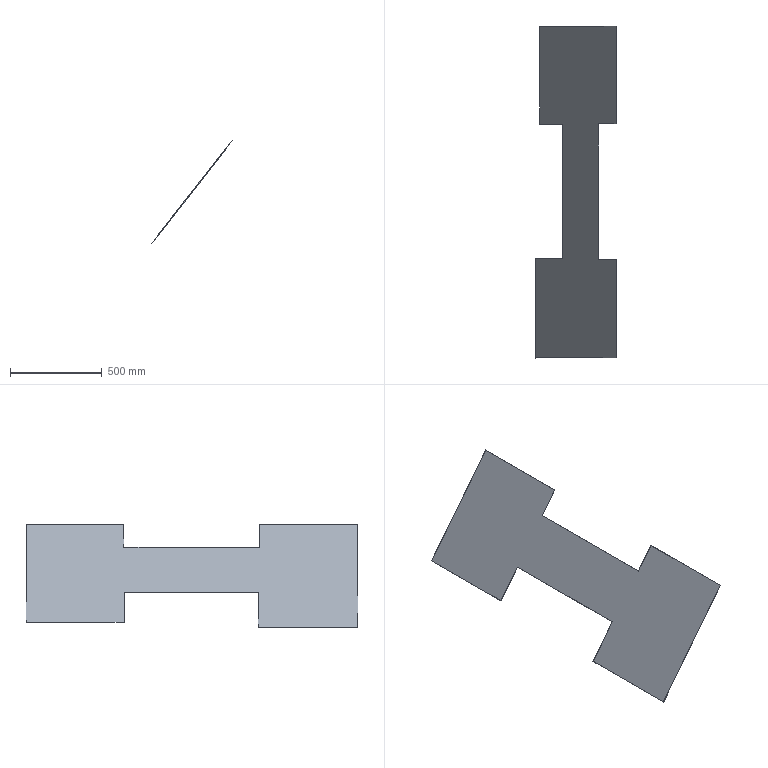Part | STEP file | fixed baffle panel | 1 solid | 14 faces | box 439.017 x 1805 x 559.044 mm | volume 1940108 mm3 | plane 14
STEP:
#1=CARTESIAN_POINT('',(0.,0.,0.));
#2=DIRECTION('',(0.,0.,1.));
#3=DIRECTION('',(1.,0.,0.));
#4=AXIS2_PLACEMENT_3D('',#1,#2,#3);
#5=CARTESIAN_POINT('',(962.42,-360.483,12.039));
#6=VERTEX_POINT('',#5);
#7=CARTESIAN_POINT('',(962.42,-902.,12.039));
#8=VERTEX_POINT('',#7);
#9=CARTESIAN_POINT('',(962.42,-360.483,12.039));
#10=DIRECTION('',(0.,-1.,0.));
#11=VECTOR('',#10,1.);
#12=LINE('',#9,#11);
#13=CARTESIAN_POINT('',(963.994,-360.483,10.805));
#14=DIRECTION('',(-0.6171,0.,-0.7869));
#15=DIRECTION('',(0.7869,0.,-0.6171));
#16=AXIS2_PLACEMENT_3D('',#13,#14,#15);
#17=PLANE('',#16);
#18=CARTESIAN_POINT('',(-2.,0.));
#19=DIRECTION('',(0.,1.));
#20=VECTOR('',#19,1.);
#21=LINE('',#18,#20);
#22=(GEOMETRIC_REPRESENTATION_CONTEXT(2)PARAMETRIC_REPRESENTATION_CONTEXT()REPRESENTATION_CONTEXT('',''));
#23=DEFINITIONAL_REPRESENTATION('',(#21),#22);
#24=PCURVE('',#17,#23);
#25=CARTESIAN_POINT('',(590.082,0.,-462.752));
#26=DIRECTION('',(-0.7869,0.,0.6171));
#27=DIRECTION('',(-0.6171,0.,-0.7869));
#28=AXIS2_PLACEMENT_3D('',#25,#26,#27);
#29=PLANE('',#28);
#30=CARTESIAN_POINT('',(-603.376,360.483));
#31=DIRECTION('',(0.,1.));
#32=VECTOR('',#31,1.);
#33=LINE('',#30,#32);
#34=(GEOMETRIC_REPRESENTATION_CONTEXT(2)PARAMETRIC_REPRESENTATION_CONTEXT()REPRESENTATION_CONTEXT('',''));
#35=DEFINITIONAL_REPRESENTATION('',(#33),#34);
#36=PCURVE('',#29,#35);
#37=SURFACE_CURVE('',#12,(#24,#36),.PCURVE_S1.);
#38=EDGE_CURVE('',#6,#8,#37,.T.);
#39=ORIENTED_EDGE('',*,*,#38,.F.);
#40=CARTESIAN_POINT('',(963.994,-360.483,10.805));
#41=VERTEX_POINT('',#40);
#42=CARTESIAN_POINT('',(963.994,-360.483,10.805));
#43=DIRECTION('',(-0.7869,0.,0.6171));
#44=VECTOR('',#43,1.);
#45=LINE('',#42,#44);
#46=CARTESIAN_POINT('',(0.,0.));
#47=DIRECTION('',(-1.,0.));
#48=VECTOR('',#47,1.);
#49=LINE('',#46,#48);
#50=(GEOMETRIC_REPRESENTATION_CONTEXT(2)PARAMETRIC_REPRESENTATION_CONTEXT()REPRESENTATION_CONTEXT('',''));
#51=DEFINITIONAL_REPRESENTATION('',(#49),#50);
#52=PCURVE('',#17,#51);
#53=CARTESIAN_POINT('',(1112.096,-360.483,199.658));
#54=DIRECTION('',(0.,1.,0.));
#55=DIRECTION('',(0.,0.,-1.));
#56=AXIS2_PLACEMENT_3D('',#53,#54,#55);
#57=PLANE('',#56);
#58=CARTESIAN_POINT('',(188.854,148.102));
#59=DIRECTION('',(-0.6171,0.7869));
#60=VECTOR('',#59,1.);
#61=LINE('',#58,#60);
#62=(GEOMETRIC_REPRESENTATION_CONTEXT(2)PARAMETRIC_REPRESENTATION_CONTEXT()REPRESENTATION_CONTEXT('',''));
#63=DEFINITIONAL_REPRESENTATION('',(#61),#62);
#64=PCURVE('',#57,#63);
#65=SURFACE_CURVE('',#45,(#52,#64),.PCURVE_S1.);
#66=EDGE_CURVE('',#41,#6,#65,.T.);
#67=ORIENTED_EDGE('',*,*,#66,.F.);
#68=CARTESIAN_POINT('',(963.994,-902.,10.805));
#69=VERTEX_POINT('',#68);
#70=CARTESIAN_POINT('',(963.994,-360.483,10.805));
#71=DIRECTION('',(0.,-1.,0.));
#72=VECTOR('',#71,1.);
#73=LINE('',#70,#72);
#74=CARTESIAN_POINT('',(0.,0.));
#75=DIRECTION('',(0.,1.));
#76=VECTOR('',#75,1.);
#77=LINE('',#74,#76);
#78=(GEOMETRIC_REPRESENTATION_CONTEXT(2)PARAMETRIC_REPRESENTATION_CONTEXT()REPRESENTATION_CONTEXT('',''));
#79=DEFINITIONAL_REPRESENTATION('',(#77),#78);
#80=PCURVE('',#17,#79);
#81=CARTESIAN_POINT('',(591.655,0.,-463.986));
#82=DIRECTION('',(-0.7869,0.,0.6171));
#83=DIRECTION('',(-0.6171,0.,-0.7869));
#84=AXIS2_PLACEMENT_3D('',#81,#82,#83);
#85=PLANE('',#84);
#86=CARTESIAN_POINT('',(-603.376,360.483));
#87=DIRECTION('',(0.,1.));
#88=VECTOR('',#87,1.);
#89=LINE('',#86,#88);
#90=(GEOMETRIC_REPRESENTATION_CONTEXT(2)PARAMETRIC_REPRESENTATION_CONTEXT()REPRESENTATION_CONTEXT('',''));
#91=DEFINITIONAL_REPRESENTATION('',(#89),#90);
#92=PCURVE('',#85,#91);
#93=SURFACE_CURVE('',#73,(#80,#92),.PCURVE_S1.);
#94=EDGE_CURVE('',#41,#69,#93,.T.);
#95=ORIENTED_EDGE('',*,*,#94,.T.);
#96=CARTESIAN_POINT('',(963.994,-902.,10.805));
#97=DIRECTION('',(-0.7869,0.,0.6171));
#98=VECTOR('',#97,1.);
#99=LINE('',#96,#98);
#100=CARTESIAN_POINT('',(0.,541.517));
#101=DIRECTION('',(-1.,0.));
#102=VECTOR('',#101,1.);
#103=LINE('',#100,#102);
#104=(GEOMETRIC_REPRESENTATION_CONTEXT(2)PARAMETRIC_REPRESENTATION_CONTEXT()REPRESENTATION_CONTEXT('',''));
#105=DEFINITIONAL_REPRESENTATION('',(#103),#104);
#106=PCURVE('',#17,#105);
#107=CARTESIAN_POINT('',(963.994,-902.,10.805));
#108=DIRECTION('',(0.,-1.,0.));
#109=DIRECTION('',(0.,0.,1.));
#110=AXIS2_PLACEMENT_3D('',#107,#108,#109);
#111=PLANE('',#110);
#112=CARTESIAN_POINT('',(0.,0.));
#113=DIRECTION('',(0.6171,0.7869));
#114=VECTOR('',#113,1.);
#115=LINE('',#112,#114);
#116=(GEOMETRIC_REPRESENTATION_CONTEXT(2)PARAMETRIC_REPRESENTATION_CONTEXT()REPRESENTATION_CONTEXT('',''));
#117=DEFINITIONAL_REPRESENTATION('',(#115),#116);
#118=PCURVE('',#111,#117);
#119=SURFACE_CURVE('',#99,(#106,#118),.PCURVE_S1.);
#120=EDGE_CURVE('',#69,#8,#119,.T.);
#121=ORIENTED_EDGE('',*,*,#120,.T.);
#122=EDGE_LOOP('',(#39,#67,#95,#121));
#123=FACE_BOUND('',#122,.T.);
#124=ADVANCED_FACE('',(#123),#17,.T.);
#125=CARTESIAN_POINT('',(1399.864,-902.,569.848));
#126=VERTEX_POINT('',#125);
#127=CARTESIAN_POINT('',(962.42,-902.,12.039));
#128=DIRECTION('',(0.6171,0.,0.7869));
#129=VECTOR('',#128,1.);
#130=LINE('',#127,#129);
#131=CARTESIAN_POINT('',(1.234,1.574));
#132=DIRECTION('',(0.7869,-0.6171));
#133=VECTOR('',#132,1.);
#134=LINE('',#131,#133);
#135=(GEOMETRIC_REPRESENTATION_CONTEXT(2)PARAMETRIC_REPRESENTATION_CONTEXT()REPRESENTATION_CONTEXT('',''));
#136=DEFINITIONAL_REPRESENTATION('',(#134),#135);
#137=PCURVE('',#111,#136);
#138=CARTESIAN_POINT('',(-603.376,902.));
#139=DIRECTION('',(-1.,0.));
#140=VECTOR('',#139,1.);
#141=LINE('',#138,#140);
#142=(GEOMETRIC_REPRESENTATION_CONTEXT(2)PARAMETRIC_REPRESENTATION_CONTEXT()REPRESENTATION_CONTEXT('',''));
#143=DEFINITIONAL_REPRESENTATION('',(#141),#142);
#144=PCURVE('',#29,#143);
#145=SURFACE_CURVE('',#130,(#137,#144),.PCURVE_S1.);
#146=EDGE_CURVE('',#8,#126,#145,.T.);
#147=ORIENTED_EDGE('',*,*,#146,.F.);
#148=ORIENTED_EDGE('',*,*,#120,.F.);
#149=CARTESIAN_POINT('',(1401.438,-902.,568.614));
#150=VERTEX_POINT('',#149);
#151=CARTESIAN_POINT('',(963.994,-902.,10.805));
#152=DIRECTION('',(0.6171,0.,0.7869));
#153=VECTOR('',#152,1.);
#154=LINE('',#151,#153);
#155=CARTESIAN_POINT('',(0.,0.));
#156=DIRECTION('',(0.7869,-0.6171));
#157=VECTOR('',#156,1.);
#158=LINE('',#155,#157);
#159=(GEOMETRIC_REPRESENTATION_CONTEXT(2)PARAMETRIC_REPRESENTATION_CONTEXT()REPRESENTATION_CONTEXT('',''));
#160=DEFINITIONAL_REPRESENTATION('',(#158),#159);
#161=PCURVE('',#111,#160);
#162=CARTESIAN_POINT('',(-603.376,902.));
#163=DIRECTION('',(-1.,0.));
#164=VECTOR('',#163,1.);
#165=LINE('',#162,#164);
#166=(GEOMETRIC_REPRESENTATION_CONTEXT(2)PARAMETRIC_REPRESENTATION_CONTEXT()REPRESENTATION_CONTEXT('',''));
#167=DEFINITIONAL_REPRESENTATION('',(#165),#166);
#168=PCURVE('',#85,#167);
#169=SURFACE_CURVE('',#154,(#161,#168),.PCURVE_S1.);
#170=EDGE_CURVE('',#69,#150,#169,.T.);
#171=ORIENTED_EDGE('',*,*,#170,.T.);
#172=CARTESIAN_POINT('',(1401.438,-902.,568.614));
#173=DIRECTION('',(-0.7869,0.,0.6171));
#174=VECTOR('',#173,1.);
#175=LINE('',#172,#174);
#176=CARTESIAN_POINT('',(557.809,-437.443));
#177=DIRECTION('',(0.6171,0.7869));
#178=VECTOR('',#177,1.);
#179=LINE('',#176,#178);
#180=(GEOMETRIC_REPRESENTATION_CONTEXT(2)PARAMETRIC_REPRESENTATION_CONTEXT()REPRESENTATION_CONTEXT('',''));
#181=DEFINITIONAL_REPRESENTATION('',(#179),#180);
#182=PCURVE('',#111,#181);
#183=CARTESIAN_POINT('',(1401.438,-902.,568.614));
#184=DIRECTION('',(0.6171,0.,0.7869));
#185=DIRECTION('',(-0.7869,0.,0.6171));
#186=AXIS2_PLACEMENT_3D('',#183,#184,#185);
#187=PLANE('',#186);
#188=CARTESIAN_POINT('',(0.,0.));
#189=DIRECTION('',(1.,0.));
#190=VECTOR('',#189,1.);
#191=LINE('',#188,#190);
#192=(GEOMETRIC_REPRESENTATION_CONTEXT(2)PARAMETRIC_REPRESENTATION_CONTEXT()REPRESENTATION_CONTEXT('',''));
#193=DEFINITIONAL_REPRESENTATION('',(#191),#192);
#194=PCURVE('',#187,#193);
#195=SURFACE_CURVE('',#175,(#182,#194),.PCURVE_S1.);
#196=EDGE_CURVE('',#150,#126,#195,.T.);
#197=ORIENTED_EDGE('',*,*,#196,.T.);
#198=EDGE_LOOP('',(#147,#148,#171,#197));
#199=FACE_BOUND('',#198,.T.);
#200=ADVANCED_FACE('',(#199),#111,.T.);
#201=CARTESIAN_POINT('',(1399.864,-368.483,569.848));
#202=VERTEX_POINT('',#201);
#203=CARTESIAN_POINT('',(1399.864,-902.,569.848));
#204=DIRECTION('',(0.,1.,0.));
#205=VECTOR('',#204,1.);
#206=LINE('',#203,#205);
#207=CARTESIAN_POINT('',(2.,0.));
#208=DIRECTION('',(0.,-1.));
#209=VECTOR('',#208,1.);
#210=LINE('',#207,#209);
#211=(GEOMETRIC_REPRESENTATION_CONTEXT(2)PARAMETRIC_REPRESENTATION_CONTEXT()REPRESENTATION_CONTEXT('',''));
#212=DEFINITIONAL_REPRESENTATION('',(#210),#211);
#213=PCURVE('',#187,#212);
#214=CARTESIAN_POINT('',(-1312.254,902.));
#215=DIRECTION('',(0.,-1.));
#216=VECTOR('',#215,1.);
#217=LINE('',#214,#216);
#218=(GEOMETRIC_REPRESENTATION_CONTEXT(2)PARAMETRIC_REPRESENTATION_CONTEXT()REPRESENTATION_CONTEXT('',''));
#219=DEFINITIONAL_REPRESENTATION('',(#217),#218);
#220=PCURVE('',#29,#219);
#221=SURFACE_CURVE('',#206,(#213,#220),.PCURVE_S1.);
#222=EDGE_CURVE('',#126,#202,#221,.T.);
#223=ORIENTED_EDGE('',*,*,#222,.F.);
#224=ORIENTED_EDGE('',*,*,#196,.F.);
#225=CARTESIAN_POINT('',(1401.438,-368.483,568.614));
#226=VERTEX_POINT('',#225);
#227=CARTESIAN_POINT('',(1401.438,-902.,568.614));
#228=DIRECTION('',(0.,1.,0.));
#229=VECTOR('',#228,1.);
#230=LINE('',#227,#229);
#231=CARTESIAN_POINT('',(0.,0.));
#232=DIRECTION('',(0.,-1.));
#233=VECTOR('',#232,1.);
#234=LINE('',#231,#233);
#235=(GEOMETRIC_REPRESENTATION_CONTEXT(2)PARAMETRIC_REPRESENTATION_CONTEXT()REPRESENTATION_CONTEXT('',''));
#236=DEFINITIONAL_REPRESENTATION('',(#234),#235);
#237=PCURVE('',#187,#236);
#238=CARTESIAN_POINT('',(-1312.254,902.));
#239=DIRECTION('',(0.,-1.));
#240=VECTOR('',#239,1.);
#241=LINE('',#238,#240);
#242=(GEOMETRIC_REPRESENTATION_CONTEXT(2)PARAMETRIC_REPRESENTATION_CONTEXT()REPRESENTATION_CONTEXT('',''));
#243=DEFINITIONAL_REPRESENTATION('',(#241),#242);
#244=PCURVE('',#85,#243);
#245=SURFACE_CURVE('',#230,(#237,#244),.PCURVE_S1.);
#246=EDGE_CURVE('',#150,#226,#245,.T.);
#247=ORIENTED_EDGE('',*,*,#246,.T.);
#248=CARTESIAN_POINT('',(1401.438,-368.483,568.614));
#249=DIRECTION('',(-0.7869,0.,0.6171));
#250=VECTOR('',#249,1.);
#251=LINE('',#248,#250);
#252=CARTESIAN_POINT('',(0.,-533.517));
#253=DIRECTION('',(1.,0.));
#254=VECTOR('',#253,1.);
#255=LINE('',#252,#254);
#256=(GEOMETRIC_REPRESENTATION_CONTEXT(2)PARAMETRIC_REPRESENTATION_CONTEXT()REPRESENTATION_CONTEXT('',''));
#257=DEFINITIONAL_REPRESENTATION('',(#255),#256);
#258=PCURVE('',#187,#257);
#259=CARTESIAN_POINT('',(1401.438,-368.483,568.614));
#260=DIRECTION('',(0.,1.,0.));
#261=DIRECTION('',(0.,0.,-1.));
#262=AXIS2_PLACEMENT_3D('',#259,#260,#261);
#263=PLANE('',#262);
#264=CARTESIAN_POINT('',(0.,0.));
#265=DIRECTION('',(-0.6171,0.7869));
#266=VECTOR('',#265,1.);
#267=LINE('',#264,#266);
#268=(GEOMETRIC_REPRESENTATION_CONTEXT(2)PARAMETRIC_REPRESENTATION_CONTEXT()REPRESENTATION_CONTEXT('',''));
#269=DEFINITIONAL_REPRESENTATION('',(#267),#268);
#270=PCURVE('',#263,#269);
#271=SURFACE_CURVE('',#251,(#258,#270),.PCURVE_S1.);
#272=EDGE_CURVE('',#226,#202,#271,.T.);
#273=ORIENTED_EDGE('',*,*,#272,.T.);
#274=EDGE_LOOP('',(#223,#224,#247,#273));
#275=FACE_BOUND('',#274,.T.);
#276=ADVANCED_FACE('',(#275),#187,.T.);
#277=CARTESIAN_POINT('',(1303.535,-368.483,447.013));
#278=VERTEX_POINT('',#277);
#279=CARTESIAN_POINT('',(1399.864,-368.483,569.848));
#280=DIRECTION('',(-0.6171,0.,-0.7869));
#281=VECTOR('',#280,1.);
#282=LINE('',#279,#281);
#283=CARTESIAN_POINT('',(-1.234,1.574));
#284=DIRECTION('',(0.7869,0.6171));
#285=VECTOR('',#284,1.);
#286=LINE('',#283,#285);
#287=(GEOMETRIC_REPRESENTATION_CONTEXT(2)PARAMETRIC_REPRESENTATION_CONTEXT()REPRESENTATION_CONTEXT('',''));
#288=DEFINITIONAL_REPRESENTATION('',(#286),#287);
#289=PCURVE('',#263,#288);
#290=CARTESIAN_POINT('',(-1312.254,368.483));
#291=DIRECTION('',(1.,0.));
#292=VECTOR('',#291,1.);
#293=LINE('',#290,#292);
#294=(GEOMETRIC_REPRESENTATION_CONTEXT(2)PARAMETRIC_REPRESENTATION_CONTEXT()REPRESENTATION_CONTEXT('',''));
#295=DEFINITIONAL_REPRESENTATION('',(#293),#294);
#296=PCURVE('',#29,#295);
#297=SURFACE_CURVE('',#282,(#289,#296),.PCURVE_S1.);
#298=EDGE_CURVE('',#202,#278,#297,.T.);
#299=ORIENTED_EDGE('',*,*,#298,.F.);
#300=ORIENTED_EDGE('',*,*,#272,.F.);
#301=CARTESIAN_POINT('',(1305.108,-368.483,445.779));
#302=VERTEX_POINT('',#301);
#303=CARTESIAN_POINT('',(1401.438,-368.483,568.614));
#304=DIRECTION('',(-0.6171,0.,-0.7869));
#305=VECTOR('',#304,1.);
#306=LINE('',#303,#305);
#307=CARTESIAN_POINT('',(0.,0.));
#308=DIRECTION('',(0.7869,0.6171));
#309=VECTOR('',#308,1.);
#310=LINE('',#307,#309);
#311=(GEOMETRIC_REPRESENTATION_CONTEXT(2)PARAMETRIC_REPRESENTATION_CONTEXT()REPRESENTATION_CONTEXT('',''));
#312=DEFINITIONAL_REPRESENTATION('',(#310),#311);
#313=PCURVE('',#263,#312);
#314=CARTESIAN_POINT('',(-1312.254,368.483));
#315=DIRECTION('',(1.,0.));
#316=VECTOR('',#315,1.);
#317=LINE('',#314,#316);
#318=(GEOMETRIC_REPRESENTATION_CONTEXT(2)PARAMETRIC_REPRESENTATION_CONTEXT()REPRESENTATION_CONTEXT('',''));
#319=DEFINITIONAL_REPRESENTATION('',(#317),#318);
#320=PCURVE('',#85,#319);
#321=SURFACE_CURVE('',#306,(#313,#320),.PCURVE_S1.);
#322=EDGE_CURVE('',#226,#302,#321,.T.);
#323=ORIENTED_EDGE('',*,*,#322,.T.);
#324=CARTESIAN_POINT('',(1305.108,-368.483,445.779));
#325=DIRECTION('',(-0.7869,0.,0.6171));
#326=VECTOR('',#325,1.);
#327=LINE('',#324,#326);
#328=CARTESIAN_POINT('',(122.835,96.329));
#329=DIRECTION('',(-0.6171,0.7869));
#330=VECTOR('',#329,1.);
#331=LINE('',#328,#330);
#332=(GEOMETRIC_REPRESENTATION_CONTEXT(2)PARAMETRIC_REPRESENTATION_CONTEXT()REPRESENTATION_CONTEXT('',''));
#333=DEFINITIONAL_REPRESENTATION('',(#331),#332);
#334=PCURVE('',#263,#333);
#335=CARTESIAN_POINT('',(1305.108,-368.483,445.779));
#336=DIRECTION('',(0.6171,0.,0.7869));
#337=DIRECTION('',(-0.7869,0.,0.6171));
#338=AXIS2_PLACEMENT_3D('',#335,#336,#337);
#339=PLANE('',#338);
#340=CARTESIAN_POINT('',(0.,0.));
#341=DIRECTION('',(1.,0.));
#342=VECTOR('',#341,1.);
#343=LINE('',#340,#342);
#344=(GEOMETRIC_REPRESENTATION_CONTEXT(2)PARAMETRIC_REPRESENTATION_CONTEXT()REPRESENTATION_CONTEXT('',''));
#345=DEFINITIONAL_REPRESENTATION('',(#343),#344);
#346=PCURVE('',#339,#345);
#347=SURFACE_CURVE('',#327,(#334,#346),.PCURVE_S1.);
#348=EDGE_CURVE('',#302,#278,#347,.T.);
#349=ORIENTED_EDGE('',*,*,#348,.T.);
#350=EDGE_LOOP('',(#299,#300,#323,#349));
#351=FACE_BOUND('',#350,.T.);
#352=ADVANCED_FACE('',(#351),#263,.T.);
#353=CARTESIAN_POINT('',(1303.535,370.79,447.013));
#354=VERTEX_POINT('',#353);
#355=CARTESIAN_POINT('',(1303.535,-368.483,447.013));
#356=DIRECTION('',(0.,1.,0.));
#357=VECTOR('',#356,1.);
#358=LINE('',#355,#357);
#359=CARTESIAN_POINT('',(2.,0.));
#360=DIRECTION('',(0.,-1.));
#361=VECTOR('',#360,1.);
#362=LINE('',#359,#361);
#363=(GEOMETRIC_REPRESENTATION_CONTEXT(2)PARAMETRIC_REPRESENTATION_CONTEXT()REPRESENTATION_CONTEXT('',''));
#364=DEFINITIONAL_REPRESENTATION('',(#362),#363);
#365=PCURVE('',#339,#364);
#366=CARTESIAN_POINT('',(-1156.152,368.483));
#367=DIRECTION('',(0.,-1.));
#368=VECTOR('',#367,1.);
#369=LINE('',#366,#368);
#370=(GEOMETRIC_REPRESENTATION_CONTEXT(2)PARAMETRIC_REPRESENTATION_CONTEXT()REPRESENTATION_CONTEXT('',''));
#371=DEFINITIONAL_REPRESENTATION('',(#369),#370);
#372=PCURVE('',#29,#371);
#373=SURFACE_CURVE('',#358,(#365,#372),.PCURVE_S1.);
#374=EDGE_CURVE('',#278,#354,#373,.T.);
#375=ORIENTED_EDGE('',*,*,#374,.F.);
#376=ORIENTED_EDGE('',*,*,#348,.F.);
#377=CARTESIAN_POINT('',(1305.108,370.79,445.779));
#378=VERTEX_POINT('',#377);
#379=CARTESIAN_POINT('',(1305.108,-368.483,445.779));
#380=DIRECTION('',(0.,1.,0.));
#381=VECTOR('',#380,1.);
#382=LINE('',#379,#381);
#383=CARTESIAN_POINT('',(0.,0.));
#384=DIRECTION('',(0.,-1.));
#385=VECTOR('',#384,1.);
#386=LINE('',#383,#385);
#387=(GEOMETRIC_REPRESENTATION_CONTEXT(2)PARAMETRIC_REPRESENTATION_CONTEXT()REPRESENTATION_CONTEXT('',''));
#388=DEFINITIONAL_REPRESENTATION('',(#386),#387);
#389=PCURVE('',#339,#388);
#390=CARTESIAN_POINT('',(-1156.152,368.483));
#391=DIRECTION('',(0.,-1.));
#392=VECTOR('',#391,1.);
#393=LINE('',#390,#392);
#394=(GEOMETRIC_REPRESENTATION_CONTEXT(2)PARAMETRIC_REPRESENTATION_CONTEXT()REPRESENTATION_CONTEXT('',''));
#395=DEFINITIONAL_REPRESENTATION('',(#393),#394);
#396=PCURVE('',#85,#395);
#397=SURFACE_CURVE('',#382,(#389,#396),.PCURVE_S1.);
#398=EDGE_CURVE('',#302,#378,#397,.T.);
#399=ORIENTED_EDGE('',*,*,#398,.T.);
#400=CARTESIAN_POINT('',(1305.108,370.79,445.779));
#401=DIRECTION('',(-0.7869,0.,0.6171));
#402=VECTOR('',#401,1.);
#403=LINE('',#400,#402);
#404=CARTESIAN_POINT('',(0.,-739.273));
#405=DIRECTION('',(1.,0.));
#406=VECTOR('',#405,1.);
#407=LINE('',#404,#406);
#408=(GEOMETRIC_REPRESENTATION_CONTEXT(2)PARAMETRIC_REPRESENTATION_CONTEXT()REPRESENTATION_CONTEXT('',''));
#409=DEFINITIONAL_REPRESENTATION('',(#407),#408);
#410=PCURVE('',#339,#409);
#411=CARTESIAN_POINT('',(1308.874,370.79,450.581));
#412=DIRECTION('',(0.,-1.,0.));
#413=DIRECTION('',(0.,0.,1.));
#414=AXIS2_PLACEMENT_3D('',#411,#412,#413);
#415=PLANE('',#414);
#416=CARTESIAN_POINT('',(-4.801,3.765));
#417=DIRECTION('',(0.6171,0.7869));
#418=VECTOR('',#417,1.);
#419=LINE('',#416,#418);
#420=(GEOMETRIC_REPRESENTATION_CONTEXT(2)PARAMETRIC_REPRESENTATION_CONTEXT()REPRESENTATION_CONTEXT('',''));
#421=DEFINITIONAL_REPRESENTATION('',(#419),#420);
#422=PCURVE('',#415,#421);
#423=SURFACE_CURVE('',#403,(#410,#422),.PCURVE_S1.);
#424=EDGE_CURVE('',#378,#354,#423,.T.);
#425=ORIENTED_EDGE('',*,*,#424,.T.);
#426=EDGE_LOOP('',(#375,#376,#399,#425));
#427=FACE_BOUND('',#426,.T.);
#428=ADVANCED_FACE('',(#427),#339,.T.);
#429=CARTESIAN_POINT('',(1399.864,370.79,569.848));
#430=VERTEX_POINT('',#429);
#431=CARTESIAN_POINT('',(1307.3,370.79,451.815));
#432=DIRECTION('',(0.6171,0.,0.7869));
#433=VECTOR('',#432,1.);
#434=LINE('',#431,#433);
#435=CARTESIAN_POINT('',(1.234,1.574));
#436=DIRECTION('',(0.7869,-0.6171));
#437=VECTOR('',#436,1.);
#438=LINE('',#435,#437);
#439=(GEOMETRIC_REPRESENTATION_CONTEXT(2)PARAMETRIC_REPRESENTATION_CONTEXT()REPRESENTATION_CONTEXT('',''));
#440=DEFINITIONAL_REPRESENTATION('',(#438),#439);
#441=PCURVE('',#415,#440);
#442=CARTESIAN_POINT('',(-1162.254,-370.79));
#443=DIRECTION('',(-1.,0.));
#444=VECTOR('',#443,1.);
#445=LINE('',#442,#444);
#446=(GEOMETRIC_REPRESENTATION_CONTEXT(2)PARAMETRIC_REPRESENTATION_CONTEXT()REPRESENTATION_CONTEXT('',''));
#447=DEFINITIONAL_REPRESENTATION('',(#445),#446);
#448=PCURVE('',#29,#447);
#449=SURFACE_CURVE('',#434,(#441,#448),.PCURVE_S1.);
#450=EDGE_CURVE('',#354,#430,#449,.T.);
#451=ORIENTED_EDGE('',*,*,#450,.F.);
#452=ORIENTED_EDGE('',*,*,#424,.F.);
#453=CARTESIAN_POINT('',(1401.438,370.79,568.614));
#454=VERTEX_POINT('',#453);
#455=CARTESIAN_POINT('',(1308.874,370.79,450.581));
#456=DIRECTION('',(0.6171,0.,0.7869));
#457=VECTOR('',#456,1.);
#458=LINE('',#455,#457);
#459=CARTESIAN_POINT('',(0.,0.));
#460=DIRECTION('',(0.7869,-0.6171));
#461=VECTOR('',#460,1.);
#462=LINE('',#459,#461);
#463=(GEOMETRIC_REPRESENTATION_CONTEXT(2)PARAMETRIC_REPRESENTATION_CONTEXT()REPRESENTATION_CONTEXT('',''));
#464=DEFINITIONAL_REPRESENTATION('',(#462),#463);
#465=PCURVE('',#415,#464);
#466=CARTESIAN_POINT('',(-1162.254,-370.79));
#467=DIRECTION('',(-1.,0.));
#468=VECTOR('',#467,1.);
#469=LINE('',#466,#468);
#470=(GEOMETRIC_REPRESENTATION_CONTEXT(2)PARAMETRIC_REPRESENTATION_CONTEXT()REPRESENTATION_CONTEXT('',''));
#471=DEFINITIONAL_REPRESENTATION('',(#469),#470);
#472=PCURVE('',#85,#471);
#473=SURFACE_CURVE('',#458,(#465,#472),.PCURVE_S1.);
#474=EDGE_CURVE('',#378,#454,#473,.T.);
#475=ORIENTED_EDGE('',*,*,#474,.T.);
#476=CARTESIAN_POINT('',(1401.438,370.79,568.614));
#477=DIRECTION('',(-0.7869,0.,0.6171));
#478=VECTOR('',#477,1.);
#479=LINE('',#476,#478);
#480=CARTESIAN_POINT('',(118.034,-92.564));
#481=DIRECTION('',(0.6171,0.7869));
#482=VECTOR('',#481,1.);
#483=LINE('',#480,#482);
#484=(GEOMETRIC_REPRESENTATION_CONTEXT(2)PARAMETRIC_REPRESENTATION_CONTEXT()REPRESENTATION_CONTEXT('',''));
#485=DEFINITIONAL_REPRESENTATION('',(#483),#484);
#486=PCURVE('',#415,#485);
#487=CARTESIAN_POINT('',(1401.438,370.79,568.614));
#488=DIRECTION('',(0.6171,0.,0.7869));
#489=DIRECTION('',(-0.7869,0.,0.6171));
#490=AXIS2_PLACEMENT_3D('',#487,#488,#489);
#491=PLANE('',#490);
#492=CARTESIAN_POINT('',(0.,0.));
#493=DIRECTION('',(1.,0.));
#494=VECTOR('',#493,1.);
#495=LINE('',#492,#494);
#496=(GEOMETRIC_REPRESENTATION_CONTEXT(2)PARAMETRIC_REPRESENTATION_CONTEXT()REPRESENTATION_CONTEXT('',''));
#497=DEFINITIONAL_REPRESENTATION('',(#495),#496);
#498=PCURVE('',#491,#497);
#499=SURFACE_CURVE('',#479,(#486,#498),.PCURVE_S1.);
#500=EDGE_CURVE('',#454,#430,#499,.T.);
#501=ORIENTED_EDGE('',*,*,#500,.T.);
#502=EDGE_LOOP('',(#451,#452,#475,#501));
#503=FACE_BOUND('',#502,.T.);
#504=ADVANCED_FACE('',(#503),#415,.T.);
#505=CARTESIAN_POINT('',(1399.864,902.79,569.848));
#506=VERTEX_POINT('',#505);
#507=CARTESIAN_POINT('',(1399.864,370.79,569.848));
#508=DIRECTION('',(0.,1.,0.));
#509=VECTOR('',#508,1.);
#510=LINE('',#507,#509);
#511=CARTESIAN_POINT('',(2.,0.));
#512=DIRECTION('',(0.,-1.));
#513=VECTOR('',#512,1.);
#514=LINE('',#511,#513);
#515=(GEOMETRIC_REPRESENTATION_CONTEXT(2)PARAMETRIC_REPRESENTATION_CONTEXT()REPRESENTATION_CONTEXT('',''));
#516=DEFINITIONAL_REPRESENTATION('',(#514),#515);
#517=PCURVE('',#491,#516);
#518=CARTESIAN_POINT('',(-1312.254,-370.79));
#519=DIRECTION('',(0.,-1.));
#520=VECTOR('',#519,1.);
#521=LINE('',#518,#520);
#522=(GEOMETRIC_REPRESENTATION_CONTEXT(2)PARAMETRIC_REPRESENTATION_CONTEXT()REPRESENTATION_CONTEXT('',''));
#523=DEFINITIONAL_REPRESENTATION('',(#521),#522);
#524=PCURVE('',#29,#523);
#525=SURFACE_CURVE('',#510,(#517,#524),.PCURVE_S1.);
#526=EDGE_CURVE('',#430,#506,#525,.T.);
#527=ORIENTED_EDGE('',*,*,#526,.F.);
#528=ORIENTED_EDGE('',*,*,#500,.F.);
#529=CARTESIAN_POINT('',(1401.438,902.79,568.614));
#530=VERTEX_POINT('',#529);
#531=CARTESIAN_POINT('',(1401.438,370.79,568.614));
#532=DIRECTION('',(0.,1.,0.));
#533=VECTOR('',#532,1.);
#534=LINE('',#531,#533);
#535=CARTESIAN_POINT('',(0.,0.));
#536=DIRECTION('',(0.,-1.));
#537=VECTOR('',#536,1.);
#538=LINE('',#535,#537);
#539=(GEOMETRIC_REPRESENTATION_CONTEXT(2)PARAMETRIC_REPRESENTATION_CONTEXT()REPRESENTATION_CONTEXT('',''));
#540=DEFINITIONAL_REPRESENTATION('',(#538),#539);
#541=PCURVE('',#491,#540);
#542=CARTESIAN_POINT('',(-1312.254,-370.79));
#543=DIRECTION('',(0.,-1.));
#544=VECTOR('',#543,1.);
#545=LINE('',#542,#544);
#546=(GEOMETRIC_REPRESENTATION_CONTEXT(2)PARAMETRIC_REPRESENTATION_CONTEXT()REPRESENTATION_CONTEXT('',''));
#547=DEFINITIONAL_REPRESENTATION('',(#545),#546);
#548=PCURVE('',#85,#547);
#549=SURFACE_CURVE('',#534,(#541,#548),.PCURVE_S1.);
#550=EDGE_CURVE('',#454,#530,#549,.T.);
#551=ORIENTED_EDGE('',*,*,#550,.T.);
#552=CARTESIAN_POINT('',(1401.438,902.79,568.614));
#553=DIRECTION('',(-0.7869,0.,0.6171));
#554=VECTOR('',#553,1.);
#555=LINE('',#552,#554);
#556=CARTESIAN_POINT('',(0.,-532.));
#557=DIRECTION('',(1.,0.));
#558=VECTOR('',#557,1.);
#559=LINE('',#556,#558);
#560=(GEOMETRIC_REPRESENTATION_CONTEXT(2)PARAMETRIC_REPRESENTATION_CONTEXT()REPRESENTATION_CONTEXT('',''));
#561=DEFINITIONAL_REPRESENTATION('',(#559),#560);
#562=PCURVE('',#491,#561);
#563=CARTESIAN_POINT('',(1401.438,902.79,568.614));
#564=DIRECTION('',(0.,1.,0.));
#565=DIRECTION('',(0.,0.,-1.));
#566=AXIS2_PLACEMENT_3D('',#563,#564,#565);
#567=PLANE('',#566);
#568=CARTESIAN_POINT('',(0.,0.));
#569=DIRECTION('',(-0.6171,0.7869));
#570=VECTOR('',#569,1.);
#571=LINE('',#568,#570);
#572=(GEOMETRIC_REPRESENTATION_CONTEXT(2)PARAMETRIC_REPRESENTATION_CONTEXT()REPRESENTATION_CONTEXT('',''));
#573=DEFINITIONAL_REPRESENTATION('',(#571),#572);
#574=PCURVE('',#567,#573);
#575=SURFACE_CURVE('',#555,(#562,#574),.PCURVE_S1.);
#576=EDGE_CURVE('',#530,#506,#575,.T.);
#577=ORIENTED_EDGE('',*,*,#576,.T.);
#578=EDGE_LOOP('',(#527,#528,#551,#577));
#579=FACE_BOUND('',#578,.T.);
#580=ADVANCED_FACE('',(#579),#491,.T.);
#581=CARTESIAN_POINT('',(984.019,902.79,39.58));
#582=VERTEX_POINT('',#581);
#583=CARTESIAN_POINT('',(1399.864,902.79,569.848));
#584=DIRECTION('',(-0.6171,0.,-0.7869));
#585=VECTOR('',#584,1.);
#586=LINE('',#583,#585);
#587=CARTESIAN_POINT('',(-1.234,1.574));
#588=DIRECTION('',(0.7869,0.6171));
#589=VECTOR('',#588,1.);
#590=LINE('',#587,#589);
#591=(GEOMETRIC_REPRESENTATION_CONTEXT(2)PARAMETRIC_REPRESENTATION_CONTEXT()REPRESENTATION_CONTEXT('',''));
#592=DEFINITIONAL_REPRESENTATION('',(#590),#591);
#593=PCURVE('',#567,#592);
#594=CARTESIAN_POINT('',(-1312.254,-902.79));
#595=DIRECTION('',(1.,0.));
#596=VECTOR('',#595,1.);
#597=LINE('',#594,#596);
#598=(GEOMETRIC_REPRESENTATION_CONTEXT(2)PARAMETRIC_REPRESENTATION_CONTEXT()REPRESENTATION_CONTEXT('',''));
#599=DEFINITIONAL_REPRESENTATION('',(#597),#598);
#600=PCURVE('',#29,#599);
#601=SURFACE_CURVE('',#586,(#593,#600),.PCURVE_S1.);
#602=EDGE_CURVE('',#506,#582,#601,.T.);
#603=ORIENTED_EDGE('',*,*,#602,.F.);
#604=ORIENTED_EDGE('',*,*,#576,.F.);
#605=CARTESIAN_POINT('',(985.592,902.79,38.346));
#606=VERTEX_POINT('',#605);
#607=CARTESIAN_POINT('',(1401.438,902.79,568.614));
#608=DIRECTION('',(-0.6171,0.,-0.7869));
#609=VECTOR('',#608,1.);
#610=LINE('',#607,#609);
#611=CARTESIAN_POINT('',(0.,0.));
#612=DIRECTION('',(0.7869,0.6171));
#613=VECTOR('',#612,1.);
#614=LINE('',#611,#613);
#615=(GEOMETRIC_REPRESENTATION_CONTEXT(2)PARAMETRIC_REPRESENTATION_CONTEXT()REPRESENTATION_CONTEXT('',''));
#616=DEFINITIONAL_REPRESENTATION('',(#614),#615);
#617=PCURVE('',#567,#616);
#618=CARTESIAN_POINT('',(-1312.254,-902.79));
#619=DIRECTION('',(1.,0.));
#620=VECTOR('',#619,1.);
#621=LINE('',#618,#620);
#622=(GEOMETRIC_REPRESENTATION_CONTEXT(2)PARAMETRIC_REPRESENTATION_CONTEXT()REPRESENTATION_CONTEXT('',''));
#623=DEFINITIONAL_REPRESENTATION('',(#621),#622);
#624=PCURVE('',#85,#623);
#625=SURFACE_CURVE('',#610,(#617,#624),.PCURVE_S1.);
#626=EDGE_CURVE('',#530,#606,#625,.T.);
#627=ORIENTED_EDGE('',*,*,#626,.T.);
#628=CARTESIAN_POINT('',(985.592,902.79,38.346));
#629=DIRECTION('',(-0.7869,0.,0.6171));
#630=VECTOR('',#629,1.);
#631=LINE('',#628,#630);
#632=CARTESIAN_POINT('',(530.268,415.845));
#633=DIRECTION('',(-0.6171,0.7869));
#634=VECTOR('',#633,1.);
#635=LINE('',#632,#634);
#636=(GEOMETRIC_REPRESENTATION_CONTEXT(2)PARAMETRIC_REPRESENTATION_CONTEXT()REPRESENTATION_CONTEXT('',''));
#637=DEFINITIONAL_REPRESENTATION('',(#635),#636);
#638=PCURVE('',#567,#637);
#639=CARTESIAN_POINT('',(985.592,902.79,38.346));
#640=DIRECTION('',(-0.6171,0.,-0.7869));
#641=DIRECTION('',(0.7869,0.,-0.6171));
#642=AXIS2_PLACEMENT_3D('',#639,#640,#641);
#643=PLANE('',#642);
#644=CARTESIAN_POINT('',(0.,0.));
#645=DIRECTION('',(-1.,0.));
#646=VECTOR('',#645,1.);
#647=LINE('',#644,#646);
#648=(GEOMETRIC_REPRESENTATION_CONTEXT(2)PARAMETRIC_REPRESENTATION_CONTEXT()REPRESENTATION_CONTEXT('',''));
#649=DEFINITIONAL_REPRESENTATION('',(#647),#648);
#650=PCURVE('',#643,#649);
#651=SURFACE_CURVE('',#631,(#638,#650),.PCURVE_S1.);
#652=EDGE_CURVE('',#606,#582,#651,.T.);
#653=ORIENTED_EDGE('',*,*,#652,.T.);
#654=EDGE_LOOP('',(#603,#604,#627,#653));
#655=FACE_BOUND('',#654,.T.);
#656=ADVANCED_FACE('',(#655),#567,.T.);
#657=CARTESIAN_POINT('',(984.019,369.79,39.58));
#658=VERTEX_POINT('',#657);
#659=CARTESIAN_POINT('',(984.019,0.,39.58));
#660=DIRECTION('',(0.,-1.,0.));
#661=VECTOR('',#660,1.);
#662=LINE('',#659,#661);
#663=CARTESIAN_POINT('',(-2.,902.79));
#664=DIRECTION('',(0.,1.));
#665=VECTOR('',#664,1.);
#666=LINE('',#663,#665);
#667=(GEOMETRIC_REPRESENTATION_CONTEXT(2)PARAMETRIC_REPRESENTATION_CONTEXT()REPRESENTATION_CONTEXT('',''));
#668=DEFINITIONAL_REPRESENTATION('',(#666),#667);
#669=PCURVE('',#643,#668);
#670=CARTESIAN_POINT('',(-638.376,0.));
#671=DIRECTION('',(0.,1.));
#672=VECTOR('',#671,1.);
#673=LINE('',#670,#672);
#674=(GEOMETRIC_REPRESENTATION_CONTEXT(2)PARAMETRIC_REPRESENTATION_CONTEXT()REPRESENTATION_CONTEXT('',''));
#675=DEFINITIONAL_REPRESENTATION('',(#673),#674);
#676=PCURVE('',#29,#675);
#677=SURFACE_CURVE('',#662,(#669,#676),.PCURVE_S1.);
#678=EDGE_CURVE('',#582,#658,#677,.T.);
#679=ORIENTED_EDGE('',*,*,#678,.F.);
#680=ORIENTED_EDGE('',*,*,#652,.F.);
#681=CARTESIAN_POINT('',(985.592,369.79,38.346));
#682=VERTEX_POINT('',#681);
#683=CARTESIAN_POINT('',(985.592,0.,38.346));
#684=DIRECTION('',(0.,-1.,0.));
#685=VECTOR('',#684,1.);
#686=LINE('',#683,#685);
#687=CARTESIAN_POINT('',(0.,902.79));
#688=DIRECTION('',(0.,1.));
#689=VECTOR('',#688,1.);
#690=LINE('',#687,#689);
#691=(GEOMETRIC_REPRESENTATION_CONTEXT(2)PARAMETRIC_REPRESENTATION_CONTEXT()REPRESENTATION_CONTEXT('',''));
#692=DEFINITIONAL_REPRESENTATION('',(#690),#691);
#693=PCURVE('',#643,#692);
#694=CARTESIAN_POINT('',(-638.376,0.));
#695=DIRECTION('',(0.,1.));
#696=VECTOR('',#695,1.);
#697=LINE('',#694,#696);
#698=(GEOMETRIC_REPRESENTATION_CONTEXT(2)PARAMETRIC_REPRESENTATION_CONTEXT()REPRESENTATION_CONTEXT('',''));
#699=DEFINITIONAL_REPRESENTATION('',(#697),#698);
#700=PCURVE('',#85,#699);
#701=SURFACE_CURVE('',#686,(#693,#700),.PCURVE_S1.);
#702=EDGE_CURVE('',#606,#682,#701,.T.);
#703=ORIENTED_EDGE('',*,*,#702,.T.);
#704=CARTESIAN_POINT('',(985.592,369.79,38.346));
#705=DIRECTION('',(-0.7869,0.,0.6171));
#706=VECTOR('',#705,1.);
#707=LINE('',#704,#706);
#708=CARTESIAN_POINT('',(0.,533.));
#709=DIRECTION('',(-1.,0.));
#710=VECTOR('',#709,1.);
#711=LINE('',#708,#710);
#712=(GEOMETRIC_REPRESENTATION_CONTEXT(2)PARAMETRIC_REPRESENTATION_CONTEXT()REPRESENTATION_CONTEXT('',''));
#713=DEFINITIONAL_REPRESENTATION('',(#711),#712);
#714=PCURVE('',#643,#713);
#715=CARTESIAN_POINT('',(973.251,369.79,22.608));
#716=DIRECTION('',(0.,-1.,0.));
#717=DIRECTION('',(0.,0.,1.));
#718=AXIS2_PLACEMENT_3D('',#715,#716,#717);
#719=PLANE('',#718);
#720=CARTESIAN_POINT('',(15.738,-12.342));
#721=DIRECTION('',(0.6171,0.7869));
#722=VECTOR('',#721,1.);
#723=LINE('',#720,#722);
#724=(GEOMETRIC_REPRESENTATION_CONTEXT(2)PARAMETRIC_REPRESENTATION_CONTEXT()REPRESENTATION_CONTEXT('',''));
#725=DEFINITIONAL_REPRESENTATION('',(#723),#724);
#726=PCURVE('',#719,#725);
#727=SURFACE_CURVE('',#707,(#714,#726),.PCURVE_S1.);
#728=EDGE_CURVE('',#682,#658,#727,.T.);
#729=ORIENTED_EDGE('',*,*,#728,.T.);
#730=EDGE_LOOP('',(#679,#680,#703,#729));
#731=FACE_BOUND('',#730,.T.);
#732=ADVANCED_FACE('',(#731),#643,.T.);
#733=CARTESIAN_POINT('',(1110.523,369.79,200.893));
#734=VERTEX_POINT('',#733);
#735=CARTESIAN_POINT('',(971.677,369.79,23.842));
#736=DIRECTION('',(0.6171,0.,0.7869));
#737=VECTOR('',#736,1.);
#738=LINE('',#735,#737);
#739=CARTESIAN_POINT('',(1.234,1.574));
#740=DIRECTION('',(0.7869,-0.6171));
#741=VECTOR('',#740,1.);
#742=LINE('',#739,#741);
#743=(GEOMETRIC_REPRESENTATION_CONTEXT(2)PARAMETRIC_REPRESENTATION_CONTEXT()REPRESENTATION_CONTEXT('',''));
#744=DEFINITIONAL_REPRESENTATION('',(#742),#743);
#745=PCURVE('',#719,#744);
#746=CARTESIAN_POINT('',(-618.376,-369.79));
#747=DIRECTION('',(-1.,0.));
#748=VECTOR('',#747,1.);
#749=LINE('',#746,#748);
#750=(GEOMETRIC_REPRESENTATION_CONTEXT(2)PARAMETRIC_REPRESENTATION_CONTEXT()REPRESENTATION_CONTEXT('',''));
#751=DEFINITIONAL_REPRESENTATION('',(#749),#750);
#752=PCURVE('',#29,#751);
#753=SURFACE_CURVE('',#738,(#745,#752),.PCURVE_S1.);
#754=EDGE_CURVE('',#658,#734,#753,.T.);
#755=ORIENTED_EDGE('',*,*,#754,.F.);
#756=ORIENTED_EDGE('',*,*,#728,.F.);
#757=CARTESIAN_POINT('',(1112.096,369.79,199.658));
#758=VERTEX_POINT('',#757);
#759=CARTESIAN_POINT('',(973.251,369.79,22.608));
#760=DIRECTION('',(0.6171,0.,0.7869));
#761=VECTOR('',#760,1.);
#762=LINE('',#759,#761);
#763=CARTESIAN_POINT('',(0.,0.));
#764=DIRECTION('',(0.7869,-0.6171));
#765=VECTOR('',#764,1.);
#766=LINE('',#763,#765);
#767=(GEOMETRIC_REPRESENTATION_CONTEXT(2)PARAMETRIC_REPRESENTATION_CONTEXT()REPRESENTATION_CONTEXT('',''));
#768=DEFINITIONAL_REPRESENTATION('',(#766),#767);
#769=PCURVE('',#719,#768);
#770=CARTESIAN_POINT('',(-618.376,-369.79));
#771=DIRECTION('',(-1.,0.));
#772=VECTOR('',#771,1.);
#773=LINE('',#770,#772);
#774=(GEOMETRIC_REPRESENTATION_CONTEXT(2)PARAMETRIC_REPRESENTATION_CONTEXT()REPRESENTATION_CONTEXT('',''));
#775=DEFINITIONAL_REPRESENTATION('',(#773),#774);
#776=PCURVE('',#85,#775);
#777=SURFACE_CURVE('',#762,(#769,#776),.PCURVE_S1.);
#778=EDGE_CURVE('',#682,#758,#777,.T.);
#779=ORIENTED_EDGE('',*,*,#778,.T.);
#780=CARTESIAN_POINT('',(1112.096,369.79,199.658));
#781=DIRECTION('',(-0.7869,0.,0.6171));
#782=VECTOR('',#781,1.);
#783=LINE('',#780,#782);
#784=CARTESIAN_POINT('',(177.05,-138.846));
#785=DIRECTION('',(0.6171,0.7869));
#786=VECTOR('',#785,1.);
#787=LINE('',#784,#786);
#788=(GEOMETRIC_REPRESENTATION_CONTEXT(2)PARAMETRIC_REPRESENTATION_CONTEXT()REPRESENTATION_CONTEXT('',''));
#789=DEFINITIONAL_REPRESENTATION('',(#787),#788);
#790=PCURVE('',#719,#789);
#791=CARTESIAN_POINT('',(1112.096,369.79,199.658));
#792=DIRECTION('',(-0.6171,0.,-0.7869));
#793=DIRECTION('',(0.7869,0.,-0.6171));
#794=AXIS2_PLACEMENT_3D('',#791,#792,#793);
#795=PLANE('',#794);
#796=CARTESIAN_POINT('',(0.,0.));
#797=DIRECTION('',(-1.,0.));
#798=VECTOR('',#797,1.);
#799=LINE('',#796,#798);
#800=(GEOMETRIC_REPRESENTATION_CONTEXT(2)PARAMETRIC_REPRESENTATION_CONTEXT()REPRESENTATION_CONTEXT('',''));
#801=DEFINITIONAL_REPRESENTATION('',(#799),#800);
#802=PCURVE('',#795,#801);
#803=SURFACE_CURVE('',#783,(#790,#802),.PCURVE_S1.);
#804=EDGE_CURVE('',#758,#734,#803,.T.);
#805=ORIENTED_EDGE('',*,*,#804,.T.);
#806=EDGE_LOOP('',(#755,#756,#779,#805));
#807=FACE_BOUND('',#806,.T.);
#808=ADVANCED_FACE('',(#807),#719,.T.);
#809=CARTESIAN_POINT('',(1110.523,-360.483,200.893));
#810=VERTEX_POINT('',#809);
#811=CARTESIAN_POINT('',(1110.523,369.79,200.893));
#812=DIRECTION('',(0.,-1.,0.));
#813=VECTOR('',#812,1.);
#814=LINE('',#811,#813);
#815=CARTESIAN_POINT('',(-2.,0.));
#816=DIRECTION('',(0.,1.));
#817=VECTOR('',#816,1.);
#818=LINE('',#815,#817);
#819=(GEOMETRIC_REPRESENTATION_CONTEXT(2)PARAMETRIC_REPRESENTATION_CONTEXT()REPRESENTATION_CONTEXT('',''));
#820=DEFINITIONAL_REPRESENTATION('',(#818),#819);
#821=PCURVE('',#795,#820);
#822=CARTESIAN_POINT('',(-843.376,-369.79));
#823=DIRECTION('',(0.,1.));
#824=VECTOR('',#823,1.);
#825=LINE('',#822,#824);
#826=(GEOMETRIC_REPRESENTATION_CONTEXT(2)PARAMETRIC_REPRESENTATION_CONTEXT()REPRESENTATION_CONTEXT('',''));
#827=DEFINITIONAL_REPRESENTATION('',(#825),#826);
#828=PCURVE('',#29,#827);
#829=SURFACE_CURVE('',#814,(#821,#828),.PCURVE_S1.);
#830=EDGE_CURVE('',#734,#810,#829,.T.);
#831=ORIENTED_EDGE('',*,*,#830,.F.);
#832=ORIENTED_EDGE('',*,*,#804,.F.);
#833=CARTESIAN_POINT('',(1112.096,-360.483,199.658));
#834=VERTEX_POINT('',#833);
#835=CARTESIAN_POINT('',(1112.096,369.79,199.658));
#836=DIRECTION('',(0.,-1.,0.));
#837=VECTOR('',#836,1.);
#838=LINE('',#835,#837);
#839=CARTESIAN_POINT('',(0.,0.));
#840=DIRECTION('',(0.,1.));
#841=VECTOR('',#840,1.);
#842=LINE('',#839,#841);
#843=(GEOMETRIC_REPRESENTATION_CONTEXT(2)PARAMETRIC_REPRESENTATION_CONTEXT()REPRESENTATION_CONTEXT('',''));
#844=DEFINITIONAL_REPRESENTATION('',(#842),#843);
#845=PCURVE('',#795,#844);
#846=CARTESIAN_POINT('',(-843.376,-369.79));
#847=DIRECTION('',(0.,1.));
#848=VECTOR('',#847,1.);
#849=LINE('',#846,#848);
#850=(GEOMETRIC_REPRESENTATION_CONTEXT(2)PARAMETRIC_REPRESENTATION_CONTEXT()REPRESENTATION_CONTEXT('',''));
#851=DEFINITIONAL_REPRESENTATION('',(#849),#850);
#852=PCURVE('',#85,#851);
#853=SURFACE_CURVE('',#838,(#845,#852),.PCURVE_S1.);
#854=EDGE_CURVE('',#758,#834,#853,.T.);
#855=ORIENTED_EDGE('',*,*,#854,.T.);
#856=CARTESIAN_POINT('',(1112.096,-360.483,199.658));
#857=DIRECTION('',(-0.7869,0.,0.6171));
#858=VECTOR('',#857,1.);
#859=LINE('',#856,#858);
#860=CARTESIAN_POINT('',(0.,730.273));
#861=DIRECTION('',(-1.,0.));
#862=VECTOR('',#861,1.);
#863=LINE('',#860,#862);
#864=(GEOMETRIC_REPRESENTATION_CONTEXT(2)PARAMETRIC_REPRESENTATION_CONTEXT()REPRESENTATION_CONTEXT('',''));
#865=DEFINITIONAL_REPRESENTATION('',(#863),#864);
#866=PCURVE('',#795,#865);
#867=CARTESIAN_POINT('',(0.,0.));
#868=DIRECTION('',(-0.6171,0.7869));
#869=VECTOR('',#868,1.);
#870=LINE('',#867,#869);
#871=(GEOMETRIC_REPRESENTATION_CONTEXT(2)PARAMETRIC_REPRESENTATION_CONTEXT()REPRESENTATION_CONTEXT('',''));
#872=DEFINITIONAL_REPRESENTATION('',(#870),#871);
#873=PCURVE('',#57,#872);
#874=SURFACE_CURVE('',#859,(#866,#873),.PCURVE_S1.);
#875=EDGE_CURVE('',#834,#810,#874,.T.);
#876=ORIENTED_EDGE('',*,*,#875,.T.);
#877=EDGE_LOOP('',(#831,#832,#855,#876));
#878=FACE_BOUND('',#877,.T.);
#879=ADVANCED_FACE('',(#878),#795,.T.);
#880=CARTESIAN_POINT('',(1110.523,-360.483,200.893));
#881=DIRECTION('',(-0.6171,0.,-0.7869));
#882=VECTOR('',#881,1.);
#883=LINE('',#880,#882);
#884=CARTESIAN_POINT('',(-1.234,1.574));
#885=DIRECTION('',(0.7869,0.6171));
#886=VECTOR('',#885,1.);
#887=LINE('',#884,#886);
#888=(GEOMETRIC_REPRESENTATION_CONTEXT(2)PARAMETRIC_REPRESENTATION_CONTEXT()REPRESENTATION_CONTEXT('',''));
#889=DEFINITIONAL_REPRESENTATION('',(#887),#888);
#890=PCURVE('',#57,#889);
#891=CARTESIAN_POINT('',(-843.376,360.483));
#892=DIRECTION('',(1.,0.));
#893=VECTOR('',#892,1.);
#894=LINE('',#891,#893);
#895=(GEOMETRIC_REPRESENTATION_CONTEXT(2)PARAMETRIC_REPRESENTATION_CONTEXT()REPRESENTATION_CONTEXT('',''));
#896=DEFINITIONAL_REPRESENTATION('',(#894),#895);
#897=PCURVE('',#29,#896);
#898=SURFACE_CURVE('',#883,(#890,#897),.PCURVE_S1.);
#899=EDGE_CURVE('',#810,#6,#898,.T.);
#900=ORIENTED_EDGE('',*,*,#899,.F.);
#901=ORIENTED_EDGE('',*,*,#875,.F.);
#902=CARTESIAN_POINT('',(1112.096,-360.483,199.658));
#903=DIRECTION('',(-0.6171,0.,-0.7869));
#904=VECTOR('',#903,1.);
#905=LINE('',#902,#904);
#906=CARTESIAN_POINT('',(0.,0.));
#907=DIRECTION('',(0.7869,0.6171));
#908=VECTOR('',#907,1.);
#909=LINE('',#906,#908);
#910=(GEOMETRIC_REPRESENTATION_CONTEXT(2)PARAMETRIC_REPRESENTATION_CONTEXT()REPRESENTATION_CONTEXT('',''));
#911=DEFINITIONAL_REPRESENTATION('',(#909),#910);
#912=PCURVE('',#57,#911);
#913=CARTESIAN_POINT('',(-843.376,360.483));
#914=DIRECTION('',(1.,0.));
#915=VECTOR('',#914,1.);
#916=LINE('',#913,#915);
#917=(GEOMETRIC_REPRESENTATION_CONTEXT(2)PARAMETRIC_REPRESENTATION_CONTEXT()REPRESENTATION_CONTEXT('',''));
#918=DEFINITIONAL_REPRESENTATION('',(#916),#917);
#919=PCURVE('',#85,#918);
#920=SURFACE_CURVE('',#905,(#912,#919),.PCURVE_S1.);
#921=EDGE_CURVE('',#834,#41,#920,.T.);
#922=ORIENTED_EDGE('',*,*,#921,.T.);
#923=ORIENTED_EDGE('',*,*,#66,.T.);
#924=EDGE_LOOP('',(#900,#901,#922,#923));
#925=FACE_BOUND('',#924,.T.);
#926=ADVANCED_FACE('',(#925),#57,.T.);
#927=ORIENTED_EDGE('',*,*,#94,.F.);
#928=ORIENTED_EDGE('',*,*,#921,.F.);
#929=ORIENTED_EDGE('',*,*,#854,.F.);
#930=ORIENTED_EDGE('',*,*,#778,.F.);
#931=ORIENTED_EDGE('',*,*,#702,.F.);
#932=ORIENTED_EDGE('',*,*,#626,.F.);
#933=ORIENTED_EDGE('',*,*,#550,.F.);
#934=ORIENTED_EDGE('',*,*,#474,.F.);
#935=ORIENTED_EDGE('',*,*,#398,.F.);
#936=ORIENTED_EDGE('',*,*,#322,.F.);
#937=ORIENTED_EDGE('',*,*,#246,.F.);
#938=ORIENTED_EDGE('',*,*,#170,.F.);
#939=EDGE_LOOP('',(#927,#928,#929,#930,#931,#932,#933,#934,#935,#936,#937,#938));
#940=FACE_BOUND('',#939,.T.);
#941=ADVANCED_FACE('',(#940),#85,.F.);
#942=ORIENTED_EDGE('',*,*,#38,.T.);
#943=ORIENTED_EDGE('',*,*,#146,.T.);
#944=ORIENTED_EDGE('',*,*,#222,.T.);
#945=ORIENTED_EDGE('',*,*,#298,.T.);
#946=ORIENTED_EDGE('',*,*,#374,.T.);
#947=ORIENTED_EDGE('',*,*,#450,.T.);
#948=ORIENTED_EDGE('',*,*,#526,.T.);
#949=ORIENTED_EDGE('',*,*,#602,.T.);
#950=ORIENTED_EDGE('',*,*,#678,.T.);
#951=ORIENTED_EDGE('',*,*,#754,.T.);
#952=ORIENTED_EDGE('',*,*,#830,.T.);
#953=ORIENTED_EDGE('',*,*,#899,.T.);
#954=EDGE_LOOP('',(#942,#943,#944,#945,#946,#947,#948,#949,#950,#951,#952,#953));
#955=FACE_BOUND('',#954,.T.);
#956=ADVANCED_FACE('',(#955),#29,.T.);
#957=CLOSED_SHELL('',(#124,#200,#276,#352,#428,#504,#580,#656,#732,#808,#879,#926,#941,#956));
#958=MANIFOLD_SOLID_BREP('',#957);
#959=(LENGTH_UNIT()NAMED_UNIT(*)SI_UNIT(.MILLI.,.METRE.));
#960=UNCERTAINTY_MEASURE_WITH_UNIT(LENGTH_MEASURE(0.0000001),#959,'','');
#961=(NAMED_UNIT(*)PLANE_ANGLE_UNIT()SI_UNIT($,.RADIAN.));
#962=(NAMED_UNIT(*)SI_UNIT($,.STERADIAN.)SOLID_ANGLE_UNIT());
#963=(GEOMETRIC_REPRESENTATION_CONTEXT(3)GLOBAL_UNCERTAINTY_ASSIGNED_CONTEXT((#960))GLOBAL_UNIT_ASSIGNED_CONTEXT((#959,#961,#962))REPRESENTATION_CONTEXT('',''));
#964=ADVANCED_BREP_SHAPE_REPRESENTATION('',(#4,#958),#963);